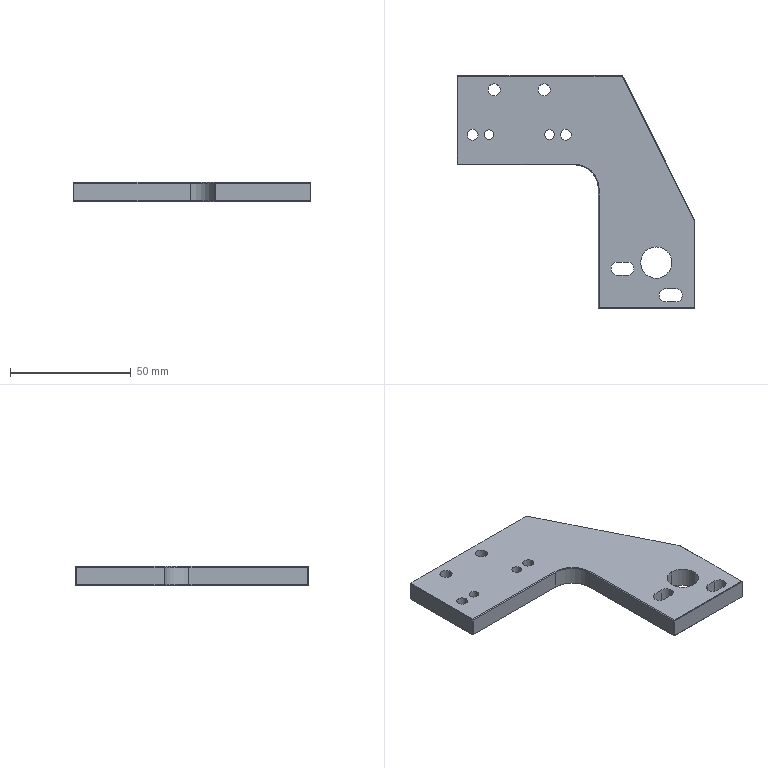Part | NX | 1 solid | 68 faces | box 98.5 x 96.5 x 8 mm | volume 38260 mm3 | plane 33 | cylinder 25 | cone 10 | commonest cylinder face diameters 5.5 x6 4 x4 4.5 x4 5 x4 8 x4 13 x2